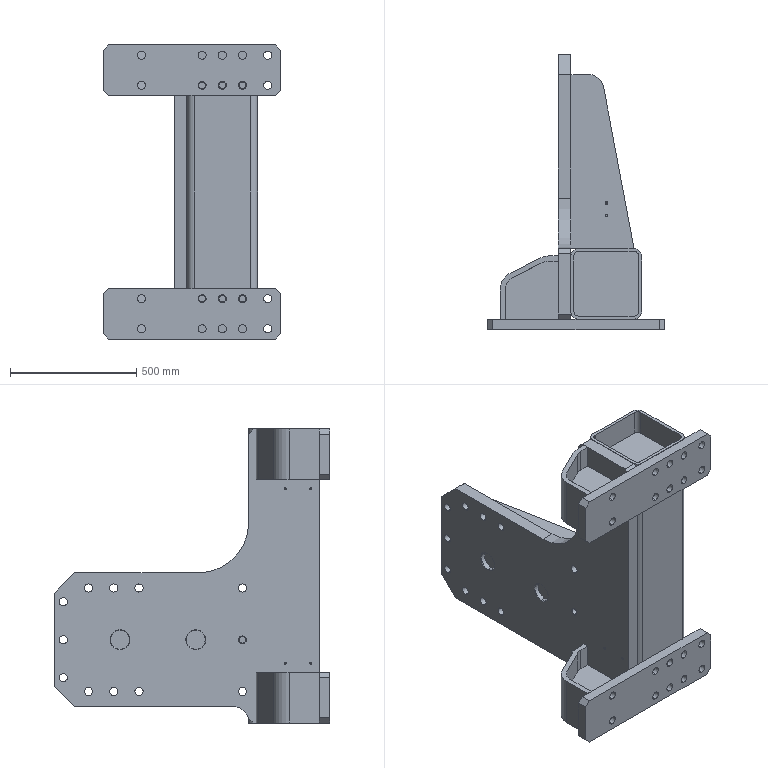Part | SolidWorks | features 3DProfileFeature 2, Cut 2, HoleWzd 2, MirrorCompFeat 2, ReferencePattern 2 | 12 solids | 330 faces | box 700 x 1090 x 1165 mm | volume 77907323 mm3 | cylinder 166 | plane 138 | cone 26 | commonest cylinder face diameters 32 x74 26.5 x26 36 x20 8.5 x12 10.2 x8 100 x8